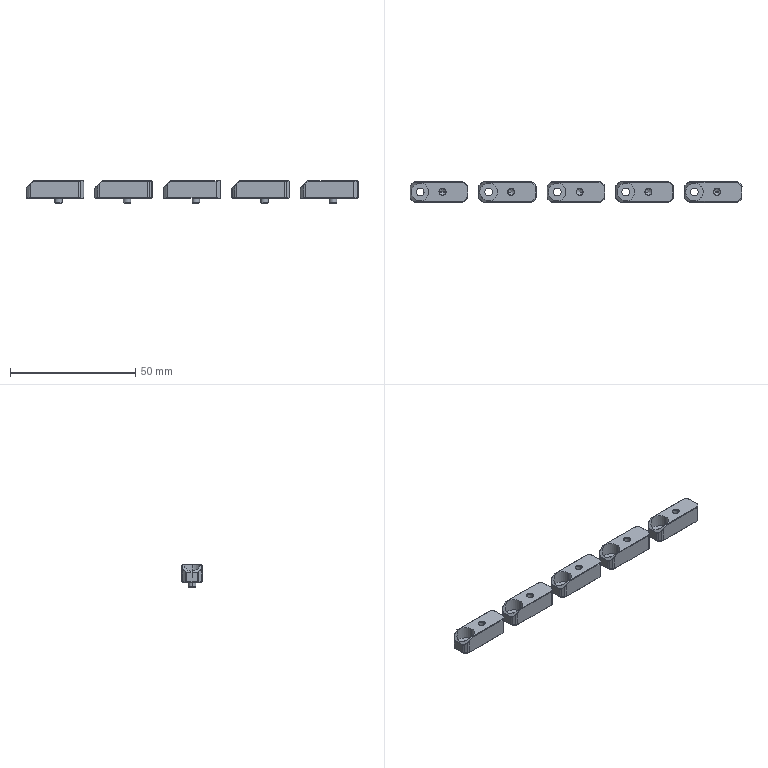Part | 5 solids | 345 faces | box 132.6 x 8 x 8.9 mm | volume 4966 mm3 | plane 155 | cone 90 | cylinder 80 | spline 20 | commonest cylinder face diameters 2 x40 2.5 x10 3 x10 3.2 x10 7 x10